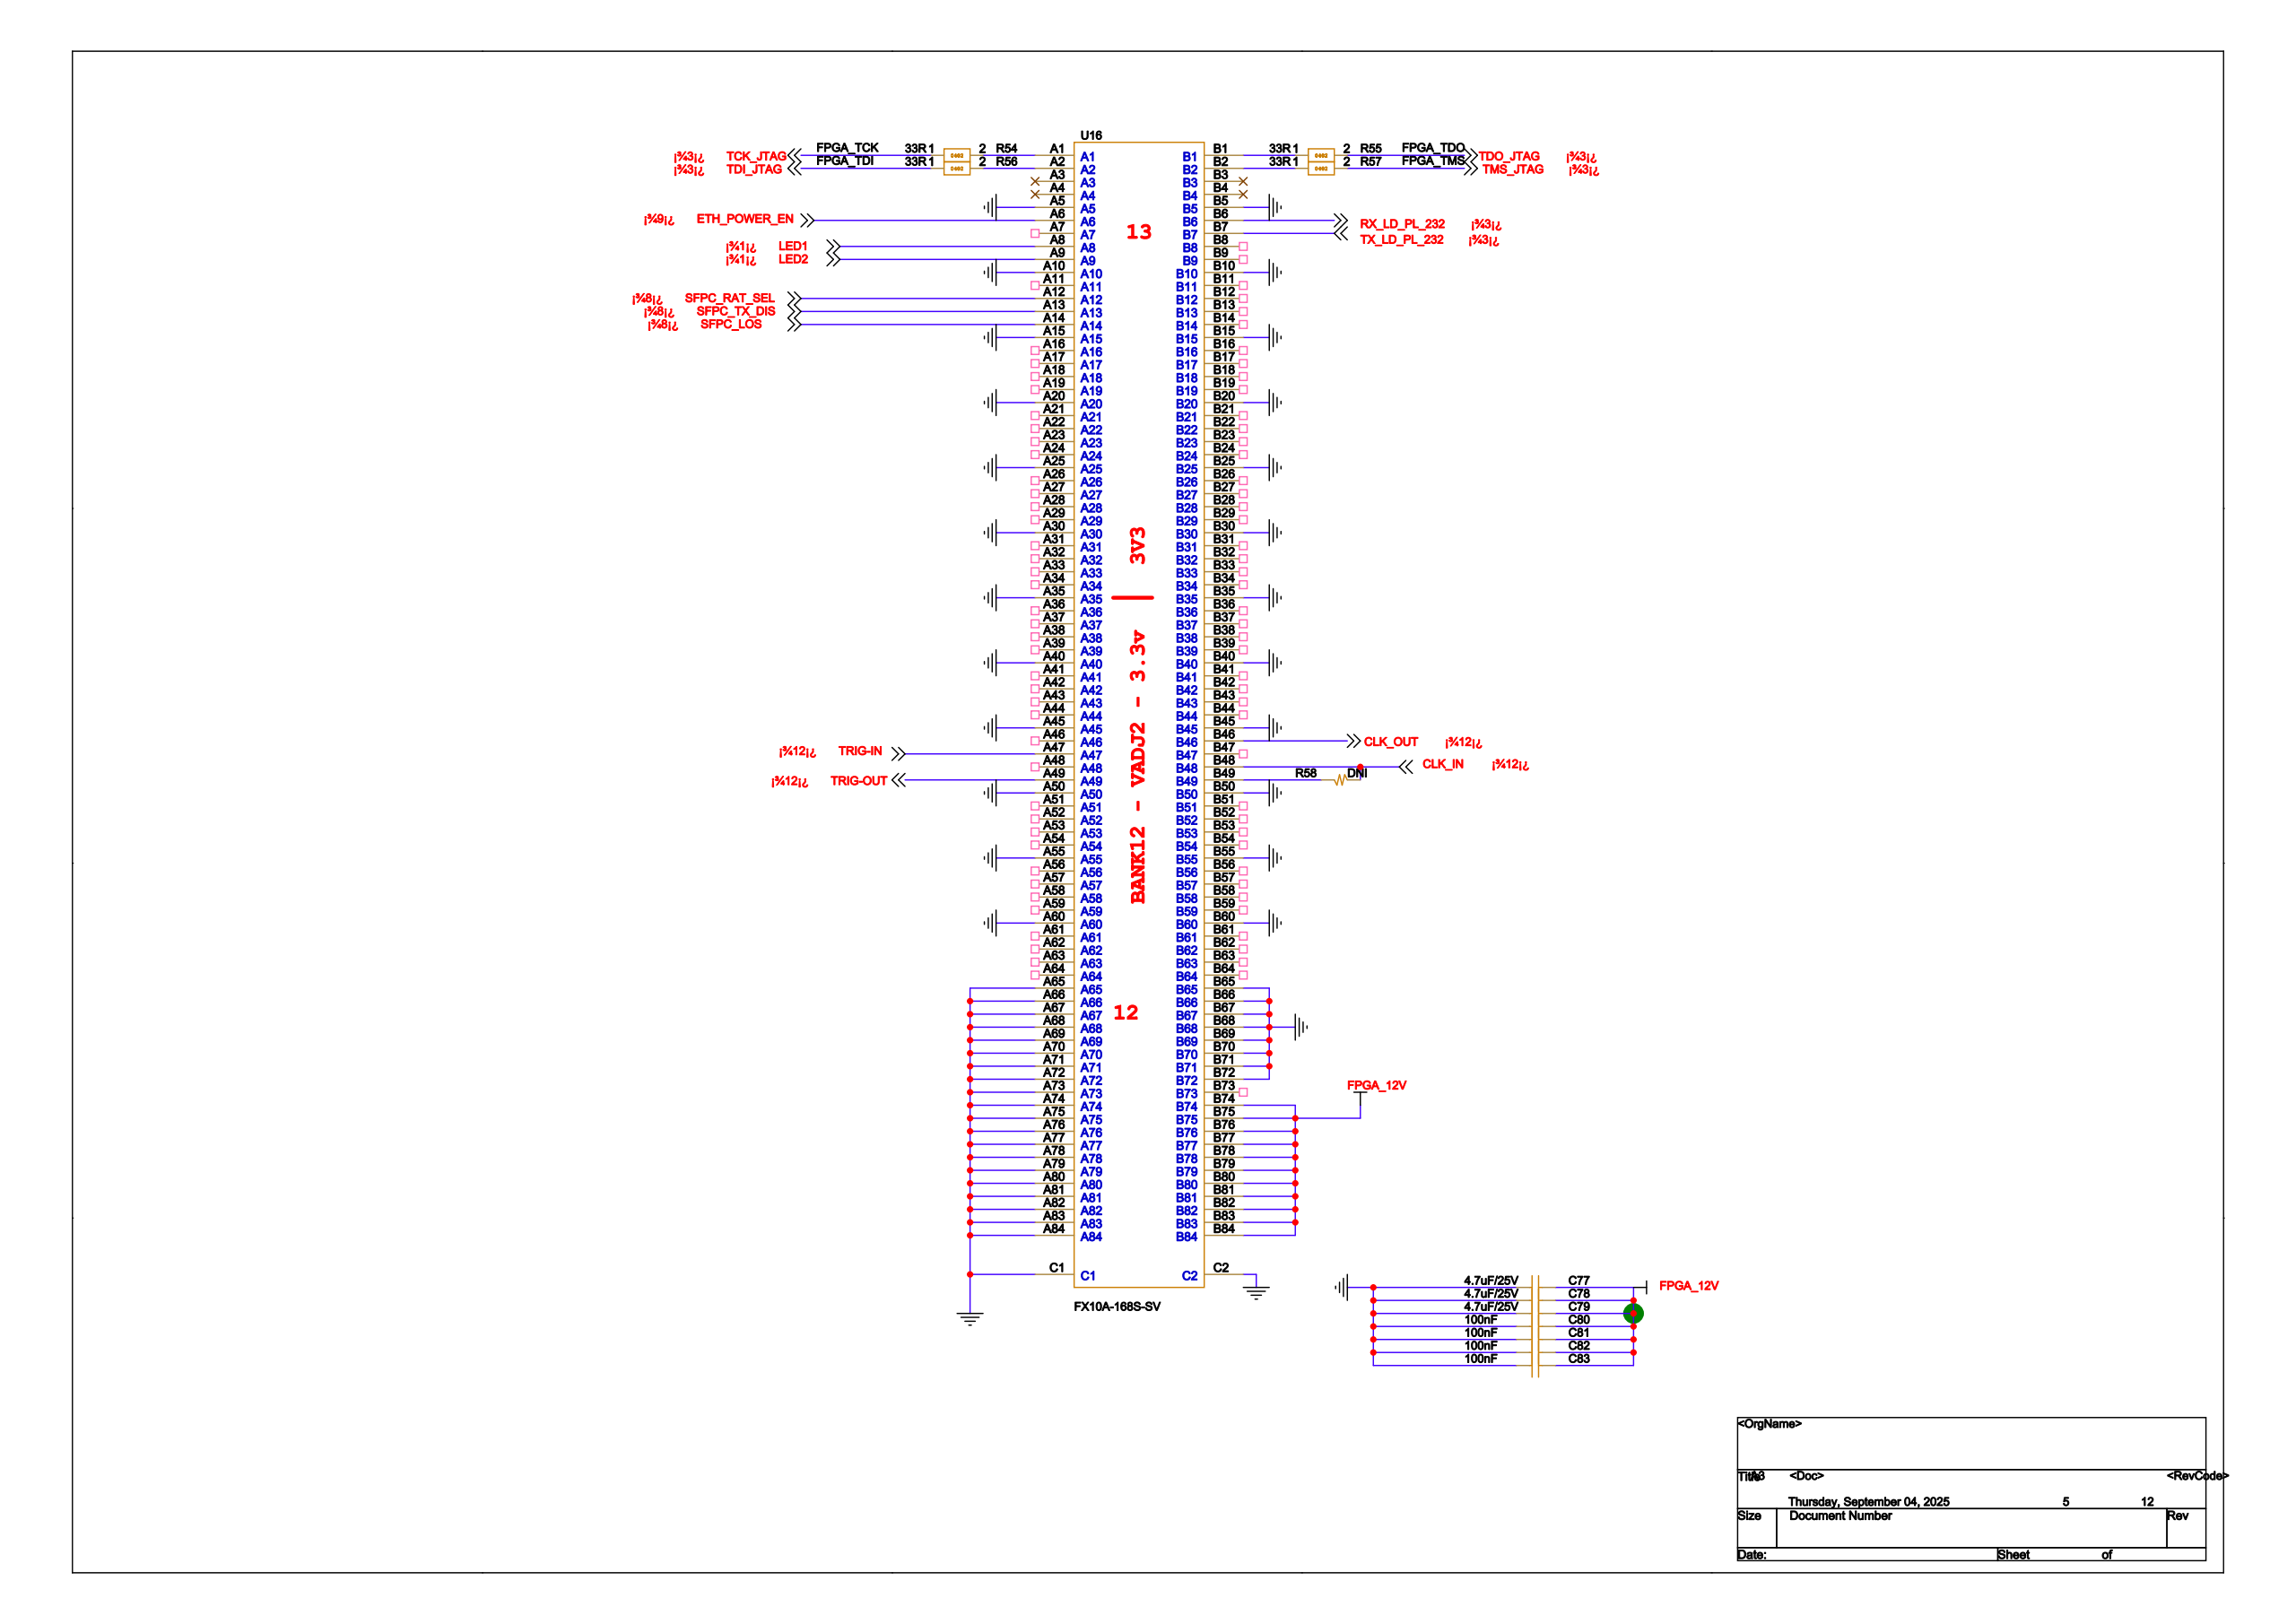Circuit board | Cadence Allegro | 528 parts | 530 nets | one sheet of the schematic
Parts on this sheet (reference | value | footprint):
C77 | 4.7uF/25V | C0603
C78 | 4.7uF/25V | C0603
C79 | 4.7uF/25V | C0603
C80 | 100nF | C0402
C81 | 100nF | C0402
C82 | 100nF | C0402
C83 | 100nF | C0402
R54 | 33R | R0402
R55 | 33R | R0402
R56 | 33R | R0402
R57 | 33R | R0402
R58 | DNI | R0402
U16 | FX10A-168S-SV | FX10A-168S-SV
Nets of these parts (net: part-pin ...):
GND: C77-1 C78-1 C79-1 C80-1 C81-1 C82-1 C83-1 U16-A5 U16-A10 U16-A15 U16-A20 U16-A25 U16-A30 U16-A35 U16-A40 U16-A45 U16-A50 U16-A55 U16-A60 U16-A65 U16-A66 U16-A67 U16-A68 U16-A69 U16-A70 U16-A71 U16-A72 U16-A73 U16-A74 U16-A75 U16-A76 U16-A77 U16-A78 U16-A79 U16-A80 U16-A81 U16-A82 U16-A83 U16-A84 U16-B5 U16-B10 U16-B15 U16-B20 U16-B25 U16-B30 U16-B35 U16-B40 U16-B45 U16-B50 U16-B55 U16-B60 U16-B65 U16-B66 U16-B67 U16-B68 U16-B69 U16-B70 U16-B71 U16-B72 U16-C1 U16-C2
CLK_IN: R58-2 U16-B48
TRIG-IN: U16-A47
CLK_OUT: U16-B46
TRIG-OUT: U16-A49
FPGA_12V: C77-2 C78-2 C79-2 C80-2 C81-2 C82-2 C83-2 U16-B74 U16-B75 U16-B76 U16-B77 U16-B78 U16-B79 U16-B80 U16-B81 U16-B82 U16-B83 U16-B84
LED1: U16-A8
LED2: U16-A9
SFPC_TX_DIS: U16-A13
SFPC_LOS: U16-A14
SFPC_RAT_SEL: U16-A12
TCK_JTAG: R54-1
TDI_JTAG: R56-1
TDO_JTAG: R55-2
TMS_JTAG: R57-2
N18158882: R54-2 U16-A1
N18157223: R55-1 U16-B1
N18158881: R56-2 U16-A2
N18157233: R57-1 U16-B2
TX_LD_PL_232: U16-B7
RX_LD_PL_232: U16-B6
N18098694: R58-1 U16-B49
ETH_POWER_EN: U16-A6